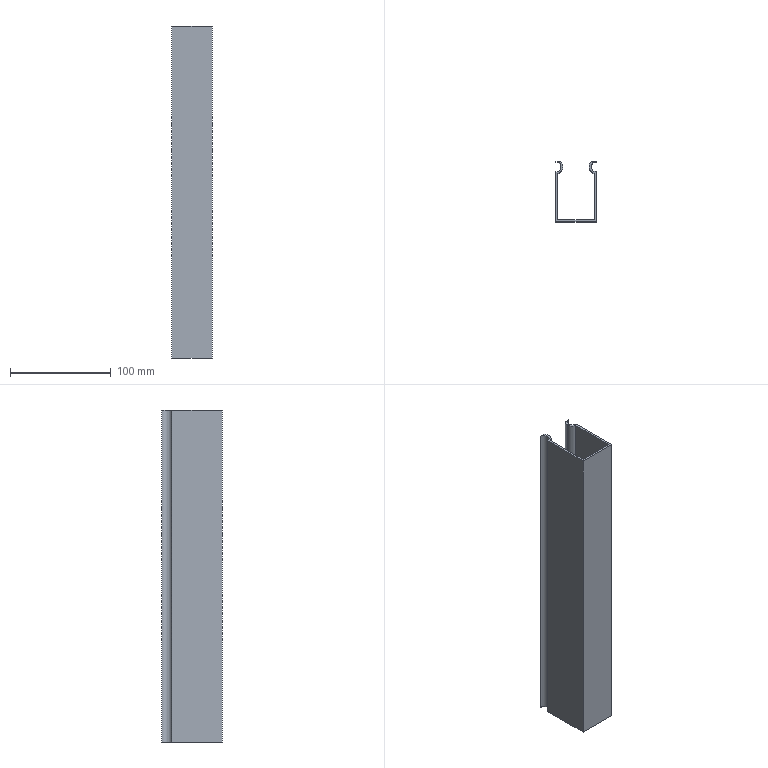Part | NX | features BREP 1 | 1 solid | 16 faces | box 40 x 60 x 330 mm | volume 107677 mm3 | plane 10 | cylinder 6 | commonest cylinder face diameters 10 x3 14 x3
STEP:
#1=CARTESIAN_POINT('',(-15.101,60.,-165.));
#2=VERTEX_POINT('',#1);
#3=CARTESIAN_POINT('',(-18.,48.292,-165.));
#4=VERTEX_POINT('',#3);
#5=CARTESIAN_POINT('',(-20.,55.,-165.));
#6=DIRECTION('',(0.,0.,-1.));
#7=DIRECTION('',(1.,0.,0.));
#8=AXIS2_PLACEMENT_3D('',#5,#6,#7);
#9=CIRCLE('',#8,7.);
#10=EDGE_CURVE('',#2,#4,#9,.T.);
#11=ORIENTED_EDGE('',*,*,#10,.F.);
#12=CARTESIAN_POINT('',(-15.101,60.,165.));
#13=VERTEX_POINT('',#12);
#14=CARTESIAN_POINT('',(-15.101,60.,165.));
#15=DIRECTION('',(0.,0.,-1.));
#16=VECTOR('',#15,1000.);
#17=LINE('',#14,#16);
#18=EDGE_CURVE('',#13,#2,#17,.T.);
#19=ORIENTED_EDGE('',*,*,#18,.F.);
#20=CARTESIAN_POINT('',(-18.,48.292,165.));
#21=VERTEX_POINT('',#20);
#22=CARTESIAN_POINT('',(-20.,55.,165.));
#23=DIRECTION('',(0.,0.,-1.));
#24=DIRECTION('',(1.,0.,0.));
#25=AXIS2_PLACEMENT_3D('',#22,#23,#24);
#26=CIRCLE('',#25,7.);
#27=EDGE_CURVE('',#13,#21,#26,.T.);
#28=ORIENTED_EDGE('',*,*,#27,.T.);
#29=CARTESIAN_POINT('',(-18.,48.292,165.));
#30=DIRECTION('',(0.,0.,-1.));
#31=VECTOR('',#30,1000.);
#32=LINE('',#29,#31);
#33=EDGE_CURVE('',#21,#4,#32,.T.);
#34=ORIENTED_EDGE('',*,*,#33,.T.);
#35=EDGE_LOOP('',(#11,#19,#28,#34));
#36=FACE_BOUND('',#35,.T.);
#37=CARTESIAN_POINT('',(-20.,55.,165.));
#38=DIRECTION('',(0.,0.,-1.));
#39=DIRECTION('',(-1.,0.,0.));
#40=AXIS2_PLACEMENT_3D('',#37,#38,#39);
#41=CYLINDRICAL_SURFACE('',#40,7.);
#42=ADVANCED_FACE('',(#36),#41,.T.);
#43=CARTESIAN_POINT('',(13.,55.,165.));
#44=VERTEX_POINT('',#43);
#45=CARTESIAN_POINT('',(13.,55.,-165.));
#46=VERTEX_POINT('',#45);
#47=CARTESIAN_POINT('',(13.,55.,165.));
#48=DIRECTION('',(0.,0.,-1.));
#49=VECTOR('',#48,1000.);
#50=LINE('',#47,#49);
#51=EDGE_CURVE('',#44,#46,#50,.T.);
#52=ORIENTED_EDGE('',*,*,#51,.F.);
#53=CARTESIAN_POINT('',(15.101,60.,165.));
#54=VERTEX_POINT('',#53);
#55=CARTESIAN_POINT('',(20.,55.,165.));
#56=DIRECTION('',(0.,0.,-1.));
#57=DIRECTION('',(1.,0.,0.));
#58=AXIS2_PLACEMENT_3D('',#55,#56,#57);
#59=CIRCLE('',#58,7.);
#60=EDGE_CURVE('',#44,#54,#59,.T.);
#61=ORIENTED_EDGE('',*,*,#60,.T.);
#62=CARTESIAN_POINT('',(15.101,60.,-165.));
#63=VERTEX_POINT('',#62);
#64=CARTESIAN_POINT('',(15.101,60.,165.));
#65=DIRECTION('',(0.,0.,-1.));
#66=VECTOR('',#65,1000.);
#67=LINE('',#64,#66);
#68=EDGE_CURVE('',#54,#63,#67,.T.);
#69=ORIENTED_EDGE('',*,*,#68,.T.);
#70=CARTESIAN_POINT('',(20.,55.,-165.));
#71=DIRECTION('',(0.,0.,-1.));
#72=DIRECTION('',(1.,0.,0.));
#73=AXIS2_PLACEMENT_3D('',#70,#71,#72);
#74=CIRCLE('',#73,7.);
#75=EDGE_CURVE('',#46,#63,#74,.T.);
#76=ORIENTED_EDGE('',*,*,#75,.F.);
#77=EDGE_LOOP('',(#52,#61,#69,#76));
#78=FACE_BOUND('',#77,.T.);
#79=CARTESIAN_POINT('',(20.,55.,165.));
#80=DIRECTION('',(0.,0.,-1.));
#81=DIRECTION('',(-1.,0.,0.));
#82=AXIS2_PLACEMENT_3D('',#79,#80,#81);
#83=CYLINDRICAL_SURFACE('',#82,7.);
#84=ADVANCED_FACE('',(#78),#83,.T.);
#85=CARTESIAN_POINT('',(18.,2.,-165.));
#86=VERTEX_POINT('',#85);
#87=CARTESIAN_POINT('',(18.,48.292,-165.));
#88=VERTEX_POINT('',#87);
#89=CARTESIAN_POINT('',(18.,0.,-165.));
#90=DIRECTION('',(0.,1.,0.));
#91=VECTOR('',#90,1000.);
#92=LINE('',#89,#91);
#93=EDGE_CURVE('',#86,#88,#92,.T.);
#94=ORIENTED_EDGE('',*,*,#93,.F.);
#95=CARTESIAN_POINT('',(18.,2.,165.));
#96=VERTEX_POINT('',#95);
#97=CARTESIAN_POINT('',(18.,2.,165.));
#98=DIRECTION('',(0.,0.,-1.));
#99=VECTOR('',#98,1000.);
#100=LINE('',#97,#99);
#101=EDGE_CURVE('',#96,#86,#100,.T.);
#102=ORIENTED_EDGE('',*,*,#101,.F.);
#103=CARTESIAN_POINT('',(18.,48.292,165.));
#104=VERTEX_POINT('',#103);
#105=CARTESIAN_POINT('',(18.,0.,165.));
#106=DIRECTION('',(0.,1.,0.));
#107=VECTOR('',#106,1000.);
#108=LINE('',#105,#107);
#109=EDGE_CURVE('',#96,#104,#108,.T.);
#110=ORIENTED_EDGE('',*,*,#109,.T.);
#111=CARTESIAN_POINT('',(18.,48.292,165.));
#112=DIRECTION('',(0.,0.,-1.));
#113=VECTOR('',#112,1000.);
#114=LINE('',#111,#113);
#115=EDGE_CURVE('',#104,#88,#114,.T.);
#116=ORIENTED_EDGE('',*,*,#115,.T.);
#117=EDGE_LOOP('',(#94,#102,#110,#116));
#118=FACE_BOUND('',#117,.T.);
#119=CARTESIAN_POINT('',(18.,0.,165.));
#120=DIRECTION('',(-1.,0.,0.));
#121=DIRECTION('',(0.,-1.,0.));
#122=AXIS2_PLACEMENT_3D('',#119,#120,#121);
#123=PLANE('',#122);
#124=ADVANCED_FACE('',(#118),#123,.T.);
#125=CARTESIAN_POINT('',(-18.,2.,-165.));
#126=VERTEX_POINT('',#125);
#127=CARTESIAN_POINT('',(20.,2.,-165.));
#128=DIRECTION('',(1.,0.,0.));
#129=VECTOR('',#128,1000.);
#130=LINE('',#127,#129);
#131=EDGE_CURVE('',#126,#86,#130,.T.);
#132=ORIENTED_EDGE('',*,*,#131,.F.);
#133=CARTESIAN_POINT('',(-18.,2.,165.));
#134=VERTEX_POINT('',#133);
#135=CARTESIAN_POINT('',(-18.,2.,165.));
#136=DIRECTION('',(0.,0.,-1.));
#137=VECTOR('',#136,1000.);
#138=LINE('',#135,#137);
#139=EDGE_CURVE('',#134,#126,#138,.T.);
#140=ORIENTED_EDGE('',*,*,#139,.F.);
#141=CARTESIAN_POINT('',(20.,2.,165.));
#142=DIRECTION('',(1.,0.,0.));
#143=VECTOR('',#142,1000.);
#144=LINE('',#141,#143);
#145=EDGE_CURVE('',#134,#96,#144,.T.);
#146=ORIENTED_EDGE('',*,*,#145,.T.);
#147=ORIENTED_EDGE('',*,*,#101,.T.);
#148=EDGE_LOOP('',(#132,#140,#146,#147));
#149=FACE_BOUND('',#148,.T.);
#150=CARTESIAN_POINT('',(20.,2.,165.));
#151=DIRECTION('',(0.,1.,0.));
#152=DIRECTION('',(0.,0.,1.));
#153=AXIS2_PLACEMENT_3D('',#150,#151,#152);
#154=PLANE('',#153);
#155=ADVANCED_FACE('',(#149),#154,.T.);
#156=CARTESIAN_POINT('',(-18.,0.,-165.));
#157=DIRECTION('',(0.,-1.,0.));
#158=VECTOR('',#157,1000.);
#159=LINE('',#156,#158);
#160=EDGE_CURVE('',#4,#126,#159,.T.);
#161=ORIENTED_EDGE('',*,*,#160,.F.);
#162=ORIENTED_EDGE('',*,*,#33,.F.);
#163=CARTESIAN_POINT('',(-18.,0.,165.));
#164=DIRECTION('',(0.,-1.,0.));
#165=VECTOR('',#164,1000.);
#166=LINE('',#163,#165);
#167=EDGE_CURVE('',#21,#134,#166,.T.);
#168=ORIENTED_EDGE('',*,*,#167,.T.);
#169=ORIENTED_EDGE('',*,*,#139,.T.);
#170=EDGE_LOOP('',(#161,#162,#168,#169));
#171=FACE_BOUND('',#170,.T.);
#172=CARTESIAN_POINT('',(-18.,0.,165.));
#173=DIRECTION('',(1.,0.,0.));
#174=DIRECTION('',(0.,1.,0.));
#175=AXIS2_PLACEMENT_3D('',#172,#173,#174);
#176=PLANE('',#175);
#177=ADVANCED_FACE('',(#171),#176,.T.);
#178=CARTESIAN_POINT('',(-20.,60.,-165.));
#179=VERTEX_POINT('',#178);
#180=CARTESIAN_POINT('',(-20.,60.,-165.));
#181=DIRECTION('',(-1.,0.,0.));
#182=VECTOR('',#181,1000.);
#183=LINE('',#180,#182);
#184=EDGE_CURVE('',#2,#179,#183,.T.);
#185=ORIENTED_EDGE('',*,*,#184,.F.);
#186=ORIENTED_EDGE('',*,*,#10,.T.);
#187=ORIENTED_EDGE('',*,*,#160,.T.);
#188=ORIENTED_EDGE('',*,*,#131,.T.);
#189=ORIENTED_EDGE('',*,*,#93,.T.);
#190=CARTESIAN_POINT('',(20.,55.,-165.));
#191=DIRECTION('',(0.,0.,-1.));
#192=DIRECTION('',(1.,0.,0.));
#193=AXIS2_PLACEMENT_3D('',#190,#191,#192);
#194=CIRCLE('',#193,7.);
#195=EDGE_CURVE('',#88,#46,#194,.T.);
#196=ORIENTED_EDGE('',*,*,#195,.T.);
#197=ORIENTED_EDGE('',*,*,#75,.T.);
#198=CARTESIAN_POINT('',(20.,60.,-165.));
#199=VERTEX_POINT('',#198);
#200=CARTESIAN_POINT('',(-20.,60.,-165.));
#201=DIRECTION('',(-1.,0.,0.));
#202=VECTOR('',#201,1000.);
#203=LINE('',#200,#202);
#204=EDGE_CURVE('',#199,#63,#203,.T.);
#205=ORIENTED_EDGE('',*,*,#204,.F.);
#206=CARTESIAN_POINT('',(15.,55.,-165.));
#207=VERTEX_POINT('',#206);
#208=CARTESIAN_POINT('',(20.,55.,-165.));
#209=DIRECTION('',(0.,0.,-1.));
#210=DIRECTION('',(-1.,0.,0.));
#211=AXIS2_PLACEMENT_3D('',#208,#209,#210);
#212=CIRCLE('',#211,5.);
#213=EDGE_CURVE('',#207,#199,#212,.T.);
#214=ORIENTED_EDGE('',*,*,#213,.F.);
#215=CARTESIAN_POINT('',(20.,50.,-165.));
#216=VERTEX_POINT('',#215);
#217=CARTESIAN_POINT('',(20.,55.,-165.));
#218=DIRECTION('',(0.,0.,-1.));
#219=DIRECTION('',(-1.,0.,0.));
#220=AXIS2_PLACEMENT_3D('',#217,#218,#219);
#221=CIRCLE('',#220,5.);
#222=EDGE_CURVE('',#216,#207,#221,.T.);
#223=ORIENTED_EDGE('',*,*,#222,.F.);
#224=CARTESIAN_POINT('',(20.,0.,-165.));
#225=VERTEX_POINT('',#224);
#226=CARTESIAN_POINT('',(20.,0.,-165.));
#227=DIRECTION('',(0.,1.,0.));
#228=VECTOR('',#227,1000.);
#229=LINE('',#226,#228);
#230=EDGE_CURVE('',#225,#216,#229,.T.);
#231=ORIENTED_EDGE('',*,*,#230,.F.);
#232=CARTESIAN_POINT('',(-20.,0.,-165.));
#233=VERTEX_POINT('',#232);
#234=CARTESIAN_POINT('',(20.,0.,-165.));
#235=DIRECTION('',(1.,0.,0.));
#236=VECTOR('',#235,1000.);
#237=LINE('',#234,#236);
#238=EDGE_CURVE('',#233,#225,#237,.T.);
#239=ORIENTED_EDGE('',*,*,#238,.F.);
#240=CARTESIAN_POINT('',(-20.,50.,-165.));
#241=VERTEX_POINT('',#240);
#242=CARTESIAN_POINT('',(-20.,0.,-165.));
#243=DIRECTION('',(0.,-1.,0.));
#244=VECTOR('',#243,1000.);
#245=LINE('',#242,#244);
#246=EDGE_CURVE('',#241,#233,#245,.T.);
#247=ORIENTED_EDGE('',*,*,#246,.F.);
#248=CARTESIAN_POINT('',(-20.,55.,-165.));
#249=DIRECTION('',(0.,0.,-1.));
#250=DIRECTION('',(1.,0.,0.));
#251=AXIS2_PLACEMENT_3D('',#248,#249,#250);
#252=CIRCLE('',#251,5.);
#253=EDGE_CURVE('',#179,#241,#252,.T.);
#254=ORIENTED_EDGE('',*,*,#253,.F.);
#255=EDGE_LOOP('',(#185,#186,#187,#188,#189,#196,#197,#205,#214,#223,#231,#239,#247,#254));
#256=FACE_BOUND('',#255,.T.);
#257=CARTESIAN_POINT('',(-20.,55.,-165.));
#258=DIRECTION('',(0.,0.,1.));
#259=DIRECTION('',(1.,0.,0.));
#260=AXIS2_PLACEMENT_3D('',#257,#258,#259);
#261=PLANE('',#260);
#262=ADVANCED_FACE('',(#256),#261,.F.);
#263=ORIENTED_EDGE('',*,*,#253,.T.);
#264=CARTESIAN_POINT('',(-20.,50.,165.));
#265=VERTEX_POINT('',#264);
#266=CARTESIAN_POINT('',(-20.,50.,165.));
#267=DIRECTION('',(0.,0.,-1.));
#268=VECTOR('',#267,1000.);
#269=LINE('',#266,#268);
#270=EDGE_CURVE('',#265,#241,#269,.T.);
#271=ORIENTED_EDGE('',*,*,#270,.F.);
#272=CARTESIAN_POINT('',(-20.,60.,165.));
#273=VERTEX_POINT('',#272);
#274=CARTESIAN_POINT('',(-20.,55.,165.));
#275=DIRECTION('',(0.,0.,-1.));
#276=DIRECTION('',(1.,0.,0.));
#277=AXIS2_PLACEMENT_3D('',#274,#275,#276);
#278=CIRCLE('',#277,5.);
#279=EDGE_CURVE('',#273,#265,#278,.T.);
#280=ORIENTED_EDGE('',*,*,#279,.F.);
#281=CARTESIAN_POINT('',(-20.,60.,165.));
#282=DIRECTION('',(0.,0.,-1.));
#283=VECTOR('',#282,1000.);
#284=LINE('',#281,#283);
#285=EDGE_CURVE('',#273,#179,#284,.T.);
#286=ORIENTED_EDGE('',*,*,#285,.T.);
#287=EDGE_LOOP('',(#263,#271,#280,#286));
#288=FACE_BOUND('',#287,.T.);
#289=CARTESIAN_POINT('',(-20.,55.,165.));
#290=DIRECTION('',(0.,0.,-1.));
#291=DIRECTION('',(-1.,0.,0.));
#292=AXIS2_PLACEMENT_3D('',#289,#290,#291);
#293=CYLINDRICAL_SURFACE('',#292,5.);
#294=ADVANCED_FACE('',(#288),#293,.F.);
#295=CARTESIAN_POINT('',(-20.,60.,165.));
#296=DIRECTION('',(-1.,0.,0.));
#297=VECTOR('',#296,1000.);
#298=LINE('',#295,#297);
#299=EDGE_CURVE('',#13,#273,#298,.T.);
#300=ORIENTED_EDGE('',*,*,#299,.F.);
#301=ORIENTED_EDGE('',*,*,#18,.T.);
#302=ORIENTED_EDGE('',*,*,#184,.T.);
#303=ORIENTED_EDGE('',*,*,#285,.F.);
#304=EDGE_LOOP('',(#300,#301,#302,#303));
#305=FACE_BOUND('',#304,.T.);
#306=CARTESIAN_POINT('',(-20.,60.,165.));
#307=DIRECTION('',(0.,-1.,0.));
#308=DIRECTION('',(0.,0.,-1.));
#309=AXIS2_PLACEMENT_3D('',#306,#307,#308);
#310=PLANE('',#309);
#311=ADVANCED_FACE('',(#305),#310,.F.);
#312=CARTESIAN_POINT('',(15.,55.,165.));
#313=VERTEX_POINT('',#312);
#314=CARTESIAN_POINT('',(15.,55.,165.));
#315=DIRECTION('',(0.,0.,-1.));
#316=VECTOR('',#315,1000.);
#317=LINE('',#314,#316);
#318=EDGE_CURVE('',#313,#207,#317,.T.);
#319=ORIENTED_EDGE('',*,*,#318,.F.);
#320=CARTESIAN_POINT('',(20.,50.,165.));
#321=VERTEX_POINT('',#320);
#322=CARTESIAN_POINT('',(20.,55.,165.));
#323=DIRECTION('',(0.,0.,-1.));
#324=DIRECTION('',(-1.,0.,0.));
#325=AXIS2_PLACEMENT_3D('',#322,#323,#324);
#326=CIRCLE('',#325,5.);
#327=EDGE_CURVE('',#321,#313,#326,.T.);
#328=ORIENTED_EDGE('',*,*,#327,.F.);
#329=CARTESIAN_POINT('',(20.,50.,165.));
#330=DIRECTION('',(0.,0.,-1.));
#331=VECTOR('',#330,1000.);
#332=LINE('',#329,#331);
#333=EDGE_CURVE('',#321,#216,#332,.T.);
#334=ORIENTED_EDGE('',*,*,#333,.T.);
#335=ORIENTED_EDGE('',*,*,#222,.T.);
#336=EDGE_LOOP('',(#319,#328,#334,#335));
#337=FACE_BOUND('',#336,.T.);
#338=CARTESIAN_POINT('',(20.,55.,165.));
#339=DIRECTION('',(0.,0.,-1.));
#340=DIRECTION('',(-1.,0.,0.));
#341=AXIS2_PLACEMENT_3D('',#338,#339,#340);
#342=CYLINDRICAL_SURFACE('',#341,5.);
#343=ADVANCED_FACE('',(#337),#342,.F.);
#344=ORIENTED_EDGE('',*,*,#230,.T.);
#345=ORIENTED_EDGE('',*,*,#333,.F.);
#346=CARTESIAN_POINT('',(20.,0.,165.));
#347=VERTEX_POINT('',#346);
#348=CARTESIAN_POINT('',(20.,0.,165.));
#349=DIRECTION('',(0.,1.,0.));
#350=VECTOR('',#349,1000.);
#351=LINE('',#348,#350);
#352=EDGE_CURVE('',#347,#321,#351,.T.);
#353=ORIENTED_EDGE('',*,*,#352,.F.);
#354=CARTESIAN_POINT('',(20.,0.,165.));
#355=DIRECTION('',(0.,0.,-1.));
#356=VECTOR('',#355,1000.);
#357=LINE('',#354,#356);
#358=EDGE_CURVE('',#347,#225,#357,.T.);
#359=ORIENTED_EDGE('',*,*,#358,.T.);
#360=EDGE_LOOP('',(#344,#345,#353,#359));
#361=FACE_BOUND('',#360,.T.);
#362=CARTESIAN_POINT('',(20.,0.,165.));
#363=DIRECTION('',(-1.,0.,0.));
#364=DIRECTION('',(0.,-1.,0.));
#365=AXIS2_PLACEMENT_3D('',#362,#363,#364);
#366=PLANE('',#365);
#367=ADVANCED_FACE('',(#361),#366,.F.);
#368=ORIENTED_EDGE('',*,*,#238,.T.);
#369=ORIENTED_EDGE('',*,*,#358,.F.);
#370=CARTESIAN_POINT('',(-20.,0.,165.));
#371=VERTEX_POINT('',#370);
#372=CARTESIAN_POINT('',(20.,0.,165.));
#373=DIRECTION('',(1.,0.,0.));
#374=VECTOR('',#373,1000.);
#375=LINE('',#372,#374);
#376=EDGE_CURVE('',#371,#347,#375,.T.);
#377=ORIENTED_EDGE('',*,*,#376,.F.);
#378=CARTESIAN_POINT('',(-20.,0.,165.));
#379=DIRECTION('',(0.,0.,-1.));
#380=VECTOR('',#379,1000.);
#381=LINE('',#378,#380);
#382=EDGE_CURVE('',#371,#233,#381,.T.);
#383=ORIENTED_EDGE('',*,*,#382,.T.);
#384=EDGE_LOOP('',(#368,#369,#377,#383));
#385=FACE_BOUND('',#384,.T.);
#386=CARTESIAN_POINT('',(20.,0.,165.));
#387=DIRECTION('',(0.,1.,0.));
#388=DIRECTION('',(0.,0.,1.));
#389=AXIS2_PLACEMENT_3D('',#386,#387,#388);
#390=PLANE('',#389);
#391=ADVANCED_FACE('',(#385),#390,.F.);
#392=ORIENTED_EDGE('',*,*,#246,.T.);
#393=ORIENTED_EDGE('',*,*,#382,.F.);
#394=CARTESIAN_POINT('',(-20.,0.,165.));
#395=DIRECTION('',(0.,-1.,0.));
#396=VECTOR('',#395,1000.);
#397=LINE('',#394,#396);
#398=EDGE_CURVE('',#265,#371,#397,.T.);
#399=ORIENTED_EDGE('',*,*,#398,.F.);
#400=ORIENTED_EDGE('',*,*,#270,.T.);
#401=EDGE_LOOP('',(#392,#393,#399,#400));
#402=FACE_BOUND('',#401,.T.);
#403=CARTESIAN_POINT('',(-20.,0.,165.));
#404=DIRECTION('',(1.,0.,0.));
#405=DIRECTION('',(0.,1.,0.));
#406=AXIS2_PLACEMENT_3D('',#403,#404,#405);
#407=PLANE('',#406);
#408=ADVANCED_FACE('',(#402),#407,.F.);
#409=CARTESIAN_POINT('',(20.,55.,165.));
#410=DIRECTION('',(0.,0.,-1.));
#411=DIRECTION('',(1.,0.,0.));
#412=AXIS2_PLACEMENT_3D('',#409,#410,#411);
#413=CIRCLE('',#412,7.);
#414=EDGE_CURVE('',#104,#44,#413,.T.);
#415=ORIENTED_EDGE('',*,*,#414,.F.);
#416=ORIENTED_EDGE('',*,*,#109,.F.);
#417=ORIENTED_EDGE('',*,*,#145,.F.);
#418=ORIENTED_EDGE('',*,*,#167,.F.);
#419=ORIENTED_EDGE('',*,*,#27,.F.);
#420=ORIENTED_EDGE('',*,*,#299,.T.);
#421=ORIENTED_EDGE('',*,*,#279,.T.);
#422=ORIENTED_EDGE('',*,*,#398,.T.);
#423=ORIENTED_EDGE('',*,*,#376,.T.);
#424=ORIENTED_EDGE('',*,*,#352,.T.);
#425=ORIENTED_EDGE('',*,*,#327,.T.);
#426=CARTESIAN_POINT('',(20.,60.,165.));
#427=VERTEX_POINT('',#426);
#428=CARTESIAN_POINT('',(20.,55.,165.));
#429=DIRECTION('',(0.,0.,-1.));
#430=DIRECTION('',(-1.,0.,0.));
#431=AXIS2_PLACEMENT_3D('',#428,#429,#430);
#432=CIRCLE('',#431,5.);
#433=EDGE_CURVE('',#313,#427,#432,.T.);
#434=ORIENTED_EDGE('',*,*,#433,.T.);
#435=CARTESIAN_POINT('',(-20.,60.,165.));
#436=DIRECTION('',(-1.,0.,0.));
#437=VECTOR('',#436,1000.);
#438=LINE('',#435,#437);
#439=EDGE_CURVE('',#427,#54,#438,.T.);
#440=ORIENTED_EDGE('',*,*,#439,.T.);
#441=ORIENTED_EDGE('',*,*,#60,.F.);
#442=EDGE_LOOP('',(#415,#416,#417,#418,#419,#420,#421,#422,#423,#424,#425,#434,#440,#441));
#443=FACE_BOUND('',#442,.T.);
#444=CARTESIAN_POINT('',(-20.,55.,165.));
#445=DIRECTION('',(0.,0.,1.));
#446=DIRECTION('',(1.,0.,0.));
#447=AXIS2_PLACEMENT_3D('',#444,#445,#446);
#448=PLANE('',#447);
#449=ADVANCED_FACE('',(#443),#448,.T.);
#450=ORIENTED_EDGE('',*,*,#68,.F.);
#451=ORIENTED_EDGE('',*,*,#439,.F.);
#452=CARTESIAN_POINT('',(20.,60.,165.));
#453=DIRECTION('',(0.,0.,-1.));
#454=VECTOR('',#453,1000.);
#455=LINE('',#452,#454);
#456=EDGE_CURVE('',#427,#199,#455,.T.);
#457=ORIENTED_EDGE('',*,*,#456,.T.);
#458=ORIENTED_EDGE('',*,*,#204,.T.);
#459=EDGE_LOOP('',(#450,#451,#457,#458));
#460=FACE_BOUND('',#459,.T.);
#461=CARTESIAN_POINT('',(-20.,60.,165.));
#462=DIRECTION('',(0.,-1.,0.));
#463=DIRECTION('',(0.,0.,-1.));
#464=AXIS2_PLACEMENT_3D('',#461,#462,#463);
#465=PLANE('',#464);
#466=ADVANCED_FACE('',(#460),#465,.F.);
#467=ORIENTED_EDGE('',*,*,#433,.F.);
#468=ORIENTED_EDGE('',*,*,#318,.T.);
#469=ORIENTED_EDGE('',*,*,#213,.T.);
#470=ORIENTED_EDGE('',*,*,#456,.F.);
#471=EDGE_LOOP('',(#467,#468,#469,#470));
#472=FACE_BOUND('',#471,.T.);
#473=CARTESIAN_POINT('',(20.,55.,165.));
#474=DIRECTION('',(0.,0.,-1.));
#475=DIRECTION('',(-1.,0.,0.));
#476=AXIS2_PLACEMENT_3D('',#473,#474,#475);
#477=CYLINDRICAL_SURFACE('',#476,5.);
#478=ADVANCED_FACE('',(#472),#477,.F.);
#479=ORIENTED_EDGE('',*,*,#414,.T.);
#480=ORIENTED_EDGE('',*,*,#51,.T.);
#481=ORIENTED_EDGE('',*,*,#195,.F.);
#482=ORIENTED_EDGE('',*,*,#115,.F.);
#483=EDGE_LOOP('',(#479,#480,#481,#482));
#484=FACE_BOUND('',#483,.T.);
#485=CARTESIAN_POINT('',(20.,55.,165.));
#486=DIRECTION('',(0.,0.,-1.));
#487=DIRECTION('',(-1.,0.,0.));
#488=AXIS2_PLACEMENT_3D('',#485,#486,#487);
#489=CYLINDRICAL_SURFACE('',#488,7.);
#490=ADVANCED_FACE('',(#484),#489,.T.);
#491=CLOSED_SHELL('',(#42,#84,#124,#155,#177,#262,#294,#311,#343,#367,#391,#408,#449,#466,#478,#490));
#492=MANIFOLD_SOLID_BREP('',#491);
#493=(LENGTH_UNIT()NAMED_UNIT(*)SI_UNIT(.MILLI.,.METRE.));
#494=UNCERTAINTY_MEASURE_WITH_UNIT(LENGTH_MEASURE(0.00001),#493,'','');
#495=(NAMED_UNIT(*)PLANE_ANGLE_UNIT()SI_UNIT($,.RADIAN.));
#496=(NAMED_UNIT(*)SI_UNIT($,.STERADIAN.)SOLID_ANGLE_UNIT());
#497=(GEOMETRIC_REPRESENTATION_CONTEXT(3)GLOBAL_UNCERTAINTY_ASSIGNED_CONTEXT((#494))GLOBAL_UNIT_ASSIGNED_CONTEXT((#493,#495,#496))REPRESENTATION_CONTEXT('',''));
#498=ADVANCED_BREP_SHAPE_REPRESENTATION('',(#492),#497);